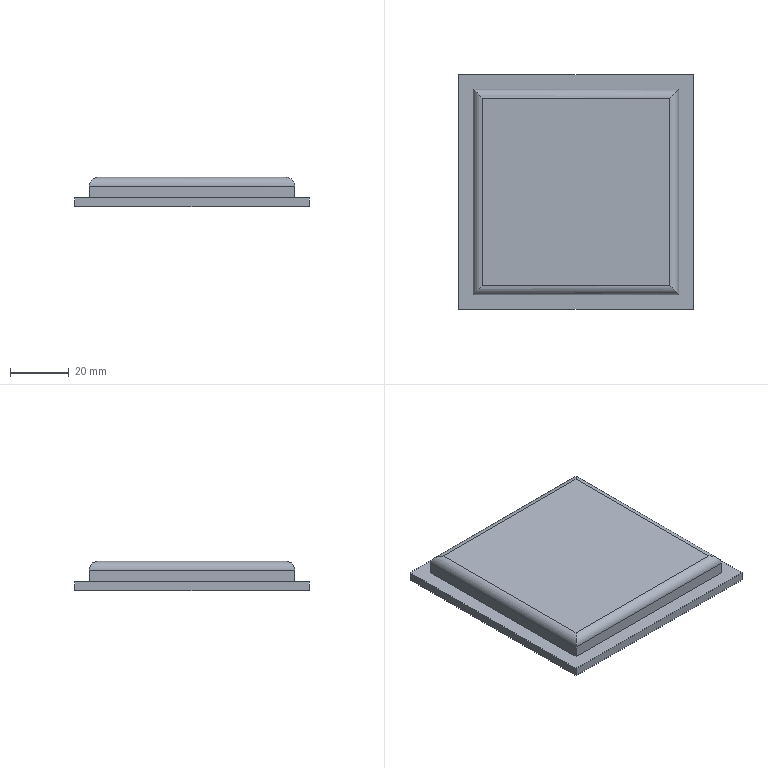Part | SolidWorks | features Extrusion 1, Fillet 1, ICE 1 | 1 solid | 15 faces | box 80 x 80 x 10 mm | volume 52970 mm3 | plane 11 | cylinder 4 | commonest cylinder face diameters 6 x4
STEP:
#1=CARTESIAN_POINT('',(40.,-40.,0.));
#2=VERTEX_POINT('',#1);
#3=CARTESIAN_POINT('',(40.,40.,0.));
#4=VERTEX_POINT('',#3);
#5=CARTESIAN_POINT('',(40.,40.,0.));
#6=DIRECTION('',(0.,1.,0.));
#7=VECTOR('',#6,1000.);
#8=LINE('',#5,#7);
#9=EDGE_CURVE('',#2,#4,#8,.T.);
#10=ORIENTED_EDGE('',*,*,#9,.T.);
#11=CARTESIAN_POINT('',(40.,40.,3.));
#12=VERTEX_POINT('',#11);
#13=CARTESIAN_POINT('',(40.,40.,3.));
#14=DIRECTION('',(0.,0.,-1.));
#15=VECTOR('',#14,1000.);
#16=LINE('',#13,#15);
#17=EDGE_CURVE('',#12,#4,#16,.T.);
#18=ORIENTED_EDGE('',*,*,#17,.F.);
#19=CARTESIAN_POINT('',(40.,-40.,3.));
#20=VERTEX_POINT('',#19);
#21=CARTESIAN_POINT('',(40.,40.,3.));
#22=DIRECTION('',(0.,1.,0.));
#23=VECTOR('',#22,1000.);
#24=LINE('',#21,#23);
#25=EDGE_CURVE('',#20,#12,#24,.T.);
#26=ORIENTED_EDGE('',*,*,#25,.F.);
#27=CARTESIAN_POINT('',(40.,-40.,3.));
#28=DIRECTION('',(0.,0.,-1.));
#29=VECTOR('',#28,1000.);
#30=LINE('',#27,#29);
#31=EDGE_CURVE('',#20,#2,#30,.T.);
#32=ORIENTED_EDGE('',*,*,#31,.T.);
#33=EDGE_LOOP('',(#10,#18,#26,#32));
#34=FACE_OUTER_BOUND('',#33,.T.);
#35=CARTESIAN_POINT('',(40.,40.,3.));
#36=DIRECTION('',(-1.,0.,0.));
#37=DIRECTION('',(0.,-1.,0.));
#38=AXIS2_PLACEMENT_3D('',#35,#36,#37);
#39=PLANE('',#38);
#40=ADVANCED_FACE('',(#34),#39,.F.);
#41=CARTESIAN_POINT('',(-40.,40.,0.));
#42=VERTEX_POINT('',#41);
#43=CARTESIAN_POINT('',(-40.,40.,0.));
#44=DIRECTION('',(-1.,0.,0.));
#45=VECTOR('',#44,1000.);
#46=LINE('',#43,#45);
#47=EDGE_CURVE('',#4,#42,#46,.T.);
#48=ORIENTED_EDGE('',*,*,#47,.T.);
#49=CARTESIAN_POINT('',(-40.,40.,3.));
#50=VERTEX_POINT('',#49);
#51=CARTESIAN_POINT('',(-40.,40.,3.));
#52=DIRECTION('',(0.,0.,-1.));
#53=VECTOR('',#52,1000.);
#54=LINE('',#51,#53);
#55=EDGE_CURVE('',#50,#42,#54,.T.);
#56=ORIENTED_EDGE('',*,*,#55,.F.);
#57=CARTESIAN_POINT('',(-40.,40.,3.));
#58=DIRECTION('',(-1.,0.,0.));
#59=VECTOR('',#58,1000.);
#60=LINE('',#57,#59);
#61=EDGE_CURVE('',#12,#50,#60,.T.);
#62=ORIENTED_EDGE('',*,*,#61,.F.);
#63=ORIENTED_EDGE('',*,*,#17,.T.);
#64=EDGE_LOOP('',(#48,#56,#62,#63));
#65=FACE_OUTER_BOUND('',#64,.T.);
#66=CARTESIAN_POINT('',(-40.,40.,3.));
#67=DIRECTION('',(0.,-1.,0.));
#68=DIRECTION('',(0.,0.,-1.));
#69=AXIS2_PLACEMENT_3D('',#66,#67,#68);
#70=PLANE('',#69);
#71=ADVANCED_FACE('',(#65),#70,.F.);
#72=CARTESIAN_POINT('',(-40.,-40.,0.));
#73=VERTEX_POINT('',#72);
#74=CARTESIAN_POINT('',(-40.,40.,0.));
#75=DIRECTION('',(0.,-1.,0.));
#76=VECTOR('',#75,1000.);
#77=LINE('',#74,#76);
#78=EDGE_CURVE('',#42,#73,#77,.T.);
#79=ORIENTED_EDGE('',*,*,#78,.T.);
#80=CARTESIAN_POINT('',(-40.,-40.,3.));
#81=VERTEX_POINT('',#80);
#82=CARTESIAN_POINT('',(-40.,-40.,3.));
#83=DIRECTION('',(0.,0.,-1.));
#84=VECTOR('',#83,1000.);
#85=LINE('',#82,#84);
#86=EDGE_CURVE('',#81,#73,#85,.T.);
#87=ORIENTED_EDGE('',*,*,#86,.F.);
#88=CARTESIAN_POINT('',(-40.,40.,3.));
#89=DIRECTION('',(0.,-1.,0.));
#90=VECTOR('',#89,1000.);
#91=LINE('',#88,#90);
#92=EDGE_CURVE('',#50,#81,#91,.T.);
#93=ORIENTED_EDGE('',*,*,#92,.F.);
#94=ORIENTED_EDGE('',*,*,#55,.T.);
#95=EDGE_LOOP('',(#79,#87,#93,#94));
#96=FACE_OUTER_BOUND('',#95,.T.);
#97=CARTESIAN_POINT('',(-40.,40.,3.));
#98=DIRECTION('',(1.,0.,0.));
#99=DIRECTION('',(0.,1.,0.));
#100=AXIS2_PLACEMENT_3D('',#97,#98,#99);
#101=PLANE('',#100);
#102=ADVANCED_FACE('',(#96),#101,.F.);
#103=CARTESIAN_POINT('',(-40.,-40.,0.));
#104=DIRECTION('',(1.,0.,0.));
#105=VECTOR('',#104,1000.);
#106=LINE('',#103,#105);
#107=EDGE_CURVE('',#73,#2,#106,.T.);
#108=ORIENTED_EDGE('',*,*,#107,.T.);
#109=ORIENTED_EDGE('',*,*,#31,.F.);
#110=CARTESIAN_POINT('',(-40.,-40.,3.));
#111=DIRECTION('',(1.,0.,0.));
#112=VECTOR('',#111,1000.);
#113=LINE('',#110,#112);
#114=EDGE_CURVE('',#81,#20,#113,.T.);
#115=ORIENTED_EDGE('',*,*,#114,.F.);
#116=ORIENTED_EDGE('',*,*,#86,.T.);
#117=EDGE_LOOP('',(#108,#109,#115,#116));
#118=FACE_OUTER_BOUND('',#117,.T.);
#119=CARTESIAN_POINT('',(-40.,-40.,3.));
#120=DIRECTION('',(0.,1.,0.));
#121=DIRECTION('',(0.,0.,1.));
#122=AXIS2_PLACEMENT_3D('',#119,#120,#121);
#123=PLANE('',#122);
#124=ADVANCED_FACE('',(#118),#123,.F.);
#125=CARTESIAN_POINT('',(35.,-35.,3.));
#126=VERTEX_POINT('',#125);
#127=CARTESIAN_POINT('',(35.,35.,3.));
#128=VERTEX_POINT('',#127);
#129=CARTESIAN_POINT('',(35.,35.,3.));
#130=DIRECTION('',(0.,1.,0.));
#131=VECTOR('',#130,1000.);
#132=LINE('',#129,#131);
#133=EDGE_CURVE('',#126,#128,#132,.T.);
#134=ORIENTED_EDGE('',*,*,#133,.F.);
#135=CARTESIAN_POINT('',(-35.,-35.,3.));
#136=VERTEX_POINT('',#135);
#137=CARTESIAN_POINT('',(-35.,-35.,3.));
#138=DIRECTION('',(1.,0.,0.));
#139=VECTOR('',#138,1000.);
#140=LINE('',#137,#139);
#141=EDGE_CURVE('',#136,#126,#140,.T.);
#142=ORIENTED_EDGE('',*,*,#141,.F.);
#143=CARTESIAN_POINT('',(-35.,35.,3.));
#144=VERTEX_POINT('',#143);
#145=CARTESIAN_POINT('',(-35.,35.,3.));
#146=DIRECTION('',(0.,-1.,0.));
#147=VECTOR('',#146,1000.);
#148=LINE('',#145,#147);
#149=EDGE_CURVE('',#144,#136,#148,.T.);
#150=ORIENTED_EDGE('',*,*,#149,.F.);
#151=CARTESIAN_POINT('',(-35.,35.,3.));
#152=DIRECTION('',(-1.,0.,0.));
#153=VECTOR('',#152,1000.);
#154=LINE('',#151,#153);
#155=EDGE_CURVE('',#128,#144,#154,.T.);
#156=ORIENTED_EDGE('',*,*,#155,.F.);
#157=EDGE_LOOP('',(#134,#142,#150,#156));
#158=FACE_BOUND('',#157,.T.);
#159=ORIENTED_EDGE('',*,*,#25,.T.);
#160=ORIENTED_EDGE('',*,*,#61,.T.);
#161=ORIENTED_EDGE('',*,*,#92,.T.);
#162=ORIENTED_EDGE('',*,*,#114,.T.);
#163=EDGE_LOOP('',(#159,#160,#161,#162));
#164=FACE_OUTER_BOUND('',#163,.T.);
#165=CARTESIAN_POINT('',(0.,0.,3.));
#166=DIRECTION('',(0.,0.,1.));
#167=DIRECTION('',(1.,0.,0.));
#168=AXIS2_PLACEMENT_3D('',#165,#166,#167);
#169=PLANE('',#168);
#170=ADVANCED_FACE('',(#158,#164),#169,.T.);
#171=ORIENTED_EDGE('',*,*,#9,.F.);
#172=ORIENTED_EDGE('',*,*,#107,.F.);
#173=ORIENTED_EDGE('',*,*,#78,.F.);
#174=ORIENTED_EDGE('',*,*,#47,.F.);
#175=EDGE_LOOP('',(#171,#172,#173,#174));
#176=FACE_OUTER_BOUND('',#175,.T.);
#177=CARTESIAN_POINT('',(0.,0.,0.));
#178=DIRECTION('',(0.,0.,1.));
#179=DIRECTION('',(1.,0.,0.));
#180=AXIS2_PLACEMENT_3D('',#177,#178,#179);
#181=PLANE('',#180);
#182=ADVANCED_FACE('',(#176),#181,.F.);
#183=CARTESIAN_POINT('',(35.,35.,7.));
#184=VERTEX_POINT('',#183);
#185=CARTESIAN_POINT('',(35.,35.,10.));
#186=DIRECTION('',(0.,0.,-1.));
#187=VECTOR('',#186,1000.);
#188=LINE('',#185,#187);
#189=EDGE_CURVE('',#184,#128,#188,.T.);
#190=ORIENTED_EDGE('',*,*,#189,.F.);
#191=CARTESIAN_POINT('',(35.,-35.,7.));
#192=VERTEX_POINT('',#191);
#193=CARTESIAN_POINT('',(35.,-35.,7.));
#194=DIRECTION('',(0.,-1.,0.));
#195=VECTOR('',#194,1000.);
#196=LINE('',#193,#195);
#197=EDGE_CURVE('',#184,#192,#196,.T.);
#198=ORIENTED_EDGE('',*,*,#197,.T.);
#199=CARTESIAN_POINT('',(35.,-35.,10.));
#200=DIRECTION('',(0.,0.,-1.));
#201=VECTOR('',#200,1000.);
#202=LINE('',#199,#201);
#203=EDGE_CURVE('',#192,#126,#202,.T.);
#204=ORIENTED_EDGE('',*,*,#203,.T.);
#205=ORIENTED_EDGE('',*,*,#133,.T.);
#206=EDGE_LOOP('',(#190,#198,#204,#205));
#207=FACE_OUTER_BOUND('',#206,.T.);
#208=CARTESIAN_POINT('',(35.,35.,10.));
#209=DIRECTION('',(-1.,0.,0.));
#210=DIRECTION('',(0.,-1.,0.));
#211=AXIS2_PLACEMENT_3D('',#208,#209,#210);
#212=PLANE('',#211);
#213=ADVANCED_FACE('',(#207),#212,.F.);
#214=CARTESIAN_POINT('',(-35.,35.,7.));
#215=VERTEX_POINT('',#214);
#216=CARTESIAN_POINT('',(-35.,35.,10.));
#217=DIRECTION('',(0.,0.,-1.));
#218=VECTOR('',#217,1000.);
#219=LINE('',#216,#218);
#220=EDGE_CURVE('',#215,#144,#219,.T.);
#221=ORIENTED_EDGE('',*,*,#220,.F.);
#222=CARTESIAN_POINT('',(35.,35.,7.));
#223=DIRECTION('',(1.,0.,0.));
#224=VECTOR('',#223,1000.);
#225=LINE('',#222,#224);
#226=EDGE_CURVE('',#215,#184,#225,.T.);
#227=ORIENTED_EDGE('',*,*,#226,.T.);
#228=ORIENTED_EDGE('',*,*,#189,.T.);
#229=ORIENTED_EDGE('',*,*,#155,.T.);
#230=EDGE_LOOP('',(#221,#227,#228,#229));
#231=FACE_OUTER_BOUND('',#230,.T.);
#232=CARTESIAN_POINT('',(-35.,35.,10.));
#233=DIRECTION('',(0.,-1.,0.));
#234=DIRECTION('',(0.,0.,-1.));
#235=AXIS2_PLACEMENT_3D('',#232,#233,#234);
#236=PLANE('',#235);
#237=ADVANCED_FACE('',(#231),#236,.F.);
#238=CARTESIAN_POINT('',(-35.,-35.,7.));
#239=VERTEX_POINT('',#238);
#240=CARTESIAN_POINT('',(-35.,-35.,10.));
#241=DIRECTION('',(0.,0.,-1.));
#242=VECTOR('',#241,1000.);
#243=LINE('',#240,#242);
#244=EDGE_CURVE('',#239,#136,#243,.T.);
#245=ORIENTED_EDGE('',*,*,#244,.F.);
#246=CARTESIAN_POINT('',(-35.,35.,7.));
#247=DIRECTION('',(0.,1.,0.));
#248=VECTOR('',#247,1000.);
#249=LINE('',#246,#248);
#250=EDGE_CURVE('',#239,#215,#249,.T.);
#251=ORIENTED_EDGE('',*,*,#250,.T.);
#252=ORIENTED_EDGE('',*,*,#220,.T.);
#253=ORIENTED_EDGE('',*,*,#149,.T.);
#254=EDGE_LOOP('',(#245,#251,#252,#253));
#255=FACE_OUTER_BOUND('',#254,.T.);
#256=CARTESIAN_POINT('',(-35.,35.,10.));
#257=DIRECTION('',(1.,0.,0.));
#258=DIRECTION('',(0.,1.,0.));
#259=AXIS2_PLACEMENT_3D('',#256,#257,#258);
#260=PLANE('',#259);
#261=ADVANCED_FACE('',(#255),#260,.F.);
#262=ORIENTED_EDGE('',*,*,#203,.F.);
#263=CARTESIAN_POINT('',(-35.,-35.,7.));
#264=DIRECTION('',(-1.,0.,0.));
#265=VECTOR('',#264,1000.);
#266=LINE('',#263,#265);
#267=EDGE_CURVE('',#192,#239,#266,.T.);
#268=ORIENTED_EDGE('',*,*,#267,.T.);
#269=ORIENTED_EDGE('',*,*,#244,.T.);
#270=ORIENTED_EDGE('',*,*,#141,.T.);
#271=EDGE_LOOP('',(#262,#268,#269,#270));
#272=FACE_OUTER_BOUND('',#271,.T.);
#273=CARTESIAN_POINT('',(-35.,-35.,10.));
#274=DIRECTION('',(0.,1.,0.));
#275=DIRECTION('',(0.,0.,1.));
#276=AXIS2_PLACEMENT_3D('',#273,#274,#275);
#277=PLANE('',#276);
#278=ADVANCED_FACE('',(#272),#277,.F.);
#279=CARTESIAN_POINT('',(-32.,32.,10.));
#280=VERTEX_POINT('',#279);
#281=CARTESIAN_POINT('',(-32.,-32.,10.));
#282=VERTEX_POINT('',#281);
#283=CARTESIAN_POINT('',(-32.,-35.,10.));
#284=DIRECTION('',(0.,-1.,0.));
#285=VECTOR('',#284,1000.);
#286=LINE('',#283,#285);
#287=EDGE_CURVE('',#280,#282,#286,.T.);
#288=ORIENTED_EDGE('',*,*,#287,.T.);
#289=CARTESIAN_POINT('',(32.,-32.,10.));
#290=VERTEX_POINT('',#289);
#291=CARTESIAN_POINT('',(35.,-32.,10.));
#292=DIRECTION('',(1.,0.,0.));
#293=VECTOR('',#292,1000.);
#294=LINE('',#291,#293);
#295=EDGE_CURVE('',#282,#290,#294,.T.);
#296=ORIENTED_EDGE('',*,*,#295,.T.);
#297=CARTESIAN_POINT('',(32.,32.,10.));
#298=VERTEX_POINT('',#297);
#299=CARTESIAN_POINT('',(32.,35.,10.));
#300=DIRECTION('',(0.,1.,0.));
#301=VECTOR('',#300,1000.);
#302=LINE('',#299,#301);
#303=EDGE_CURVE('',#290,#298,#302,.T.);
#304=ORIENTED_EDGE('',*,*,#303,.T.);
#305=CARTESIAN_POINT('',(-35.,32.,10.));
#306=DIRECTION('',(-1.,0.,0.));
#307=VECTOR('',#306,1000.);
#308=LINE('',#305,#307);
#309=EDGE_CURVE('',#298,#280,#308,.T.);
#310=ORIENTED_EDGE('',*,*,#309,.T.);
#311=EDGE_LOOP('',(#288,#296,#304,#310));
#312=FACE_OUTER_BOUND('',#311,.T.);
#313=CARTESIAN_POINT('',(0.,0.,10.));
#314=DIRECTION('',(0.,0.,1.));
#315=DIRECTION('',(1.,0.,0.));
#316=AXIS2_PLACEMENT_3D('',#313,#314,#315);
#317=PLANE('',#316);
#318=ADVANCED_FACE('',(#312),#317,.T.);
#319=CARTESIAN_POINT('',(35.,35.,7.));
#320=CARTESIAN_POINT('',(35.,35.,8.757));
#321=CARTESIAN_POINT('',(33.757,33.757,10.));
#322=CARTESIAN_POINT('',(32.,32.,10.));
#323=(BOUNDED_CURVE()B_SPLINE_CURVE(3,(#319,#320,#321,#322),.UNSPECIFIED.,.F.,.F.)B_SPLINE_CURVE_WITH_KNOTS((4,4),(3.142,4.712),.UNSPECIFIED.)CURVE()GEOMETRIC_REPRESENTATION_ITEM()RATIONAL_B_SPLINE_CURVE((1.,0.8047,0.8047,1.))REPRESENTATION_ITEM(''));
#324=EDGE_CURVE('',#184,#298,#323,.T.);
#325=ORIENTED_EDGE('',*,*,#324,.F.);
#326=ORIENTED_EDGE('',*,*,#226,.F.);
#327=CARTESIAN_POINT('',(-32.,32.,10.));
#328=CARTESIAN_POINT('',(-33.757,33.757,10.));
#329=CARTESIAN_POINT('',(-35.,35.,8.757));
#330=CARTESIAN_POINT('',(-35.,35.,7.));
#331=(BOUNDED_CURVE()B_SPLINE_CURVE(3,(#327,#328,#329,#330),.UNSPECIFIED.,.F.,.F.)B_SPLINE_CURVE_WITH_KNOTS((4,4),(1.571,3.142),.UNSPECIFIED.)CURVE()GEOMETRIC_REPRESENTATION_ITEM()RATIONAL_B_SPLINE_CURVE((1.,0.8047,0.8047,1.))REPRESENTATION_ITEM(''));
#332=EDGE_CURVE('',#280,#215,#331,.T.);
#333=ORIENTED_EDGE('',*,*,#332,.F.);
#334=ORIENTED_EDGE('',*,*,#309,.F.);
#335=EDGE_LOOP('',(#325,#326,#333,#334));
#336=FACE_OUTER_BOUND('',#335,.T.);
#337=CARTESIAN_POINT('',(0.,32.,7.));
#338=DIRECTION('',(1.,0.,0.));
#339=DIRECTION('',(0.,0.,-1.));
#340=AXIS2_PLACEMENT_3D('',#337,#338,#339);
#341=CYLINDRICAL_SURFACE('',#340,3.);
#342=ADVANCED_FACE('',(#336),#341,.T.);
#343=ORIENTED_EDGE('',*,*,#332,.T.);
#344=ORIENTED_EDGE('',*,*,#250,.F.);
#345=CARTESIAN_POINT('',(-32.,-32.,10.));
#346=CARTESIAN_POINT('',(-33.757,-33.757,10.));
#347=CARTESIAN_POINT('',(-35.,-35.,8.757));
#348=CARTESIAN_POINT('',(-35.,-35.,7.));
#349=(BOUNDED_CURVE()B_SPLINE_CURVE(3,(#345,#346,#347,#348),.UNSPECIFIED.,.F.,.F.)B_SPLINE_CURVE_WITH_KNOTS((4,4),(1.571,3.142),.UNSPECIFIED.)CURVE()GEOMETRIC_REPRESENTATION_ITEM()RATIONAL_B_SPLINE_CURVE((1.,0.8047,0.8047,1.))REPRESENTATION_ITEM(''));
#350=EDGE_CURVE('',#282,#239,#349,.T.);
#351=ORIENTED_EDGE('',*,*,#350,.F.);
#352=ORIENTED_EDGE('',*,*,#287,.F.);
#353=EDGE_LOOP('',(#343,#344,#351,#352));
#354=FACE_OUTER_BOUND('',#353,.T.);
#355=CARTESIAN_POINT('',(-32.,0.,7.));
#356=DIRECTION('',(0.,1.,0.));
#357=DIRECTION('',(-1.,0.,0.));
#358=AXIS2_PLACEMENT_3D('',#355,#356,#357);
#359=CYLINDRICAL_SURFACE('',#358,3.);
#360=ADVANCED_FACE('',(#354),#359,.T.);
#361=ORIENTED_EDGE('',*,*,#324,.T.);
#362=ORIENTED_EDGE('',*,*,#303,.F.);
#363=CARTESIAN_POINT('',(35.,-35.,7.));
#364=CARTESIAN_POINT('',(35.,-35.,8.757));
#365=CARTESIAN_POINT('',(33.757,-33.757,10.));
#366=CARTESIAN_POINT('',(32.,-32.,10.));
#367=(BOUNDED_CURVE()B_SPLINE_CURVE(3,(#363,#364,#365,#366),.UNSPECIFIED.,.F.,.F.)B_SPLINE_CURVE_WITH_KNOTS((4,4),(0.,1.571),.UNSPECIFIED.)CURVE()GEOMETRIC_REPRESENTATION_ITEM()RATIONAL_B_SPLINE_CURVE((1.,0.8047,0.8047,1.))REPRESENTATION_ITEM(''));
#368=EDGE_CURVE('',#192,#290,#367,.T.);
#369=ORIENTED_EDGE('',*,*,#368,.F.);
#370=ORIENTED_EDGE('',*,*,#197,.F.);
#371=EDGE_LOOP('',(#361,#362,#369,#370));
#372=FACE_OUTER_BOUND('',#371,.T.);
#373=CARTESIAN_POINT('',(32.,0.,7.));
#374=DIRECTION('',(0.,-1.,0.));
#375=DIRECTION('',(1.,0.,0.));
#376=AXIS2_PLACEMENT_3D('',#373,#374,#375);
#377=CYLINDRICAL_SURFACE('',#376,3.);
#378=ADVANCED_FACE('',(#372),#377,.T.);
#379=ORIENTED_EDGE('',*,*,#350,.T.);
#380=ORIENTED_EDGE('',*,*,#267,.F.);
#381=ORIENTED_EDGE('',*,*,#368,.T.);
#382=ORIENTED_EDGE('',*,*,#295,.F.);
#383=EDGE_LOOP('',(#379,#380,#381,#382));
#384=FACE_OUTER_BOUND('',#383,.T.);
#385=CARTESIAN_POINT('',(0.,-32.,7.));
#386=DIRECTION('',(-1.,0.,0.));
#387=DIRECTION('',(0.,0.,1.));
#388=AXIS2_PLACEMENT_3D('',#385,#386,#387);
#389=CYLINDRICAL_SURFACE('',#388,3.);
#390=ADVANCED_FACE('',(#384),#389,.T.);
#391=CLOSED_SHELL('',(#40,#71,#102,#124,#170,#182,#213,#237,#261,#278,#318,#342,#360,#378,#390));
#392=MANIFOLD_SOLID_BREP('',#391);
#393=CARTESIAN_POINT('',(0.,0.,0.));
#394=DIRECTION('',(0.,0.,1.));
#395=DIRECTION('',(1.,0.,0.));
#396=AXIS2_PLACEMENT_3D('',#393,#394,#395);
#397=(LENGTH_UNIT()NAMED_UNIT(*)SI_UNIT(.MILLI.,.METRE.));
#398=UNCERTAINTY_MEASURE_WITH_UNIT(LENGTH_MEASURE(0.00001),#397,'','');
#399=(NAMED_UNIT(*)PLANE_ANGLE_UNIT()SI_UNIT($,.RADIAN.));
#400=(NAMED_UNIT(*)SI_UNIT($,.STERADIAN.)SOLID_ANGLE_UNIT());
#401=(GEOMETRIC_REPRESENTATION_CONTEXT(3)GLOBAL_UNCERTAINTY_ASSIGNED_CONTEXT((#398))GLOBAL_UNIT_ASSIGNED_CONTEXT((#397,#399,#400))REPRESENTATION_CONTEXT('',''));
#402=ADVANCED_BREP_SHAPE_REPRESENTATION('',(#392,#396),#401);